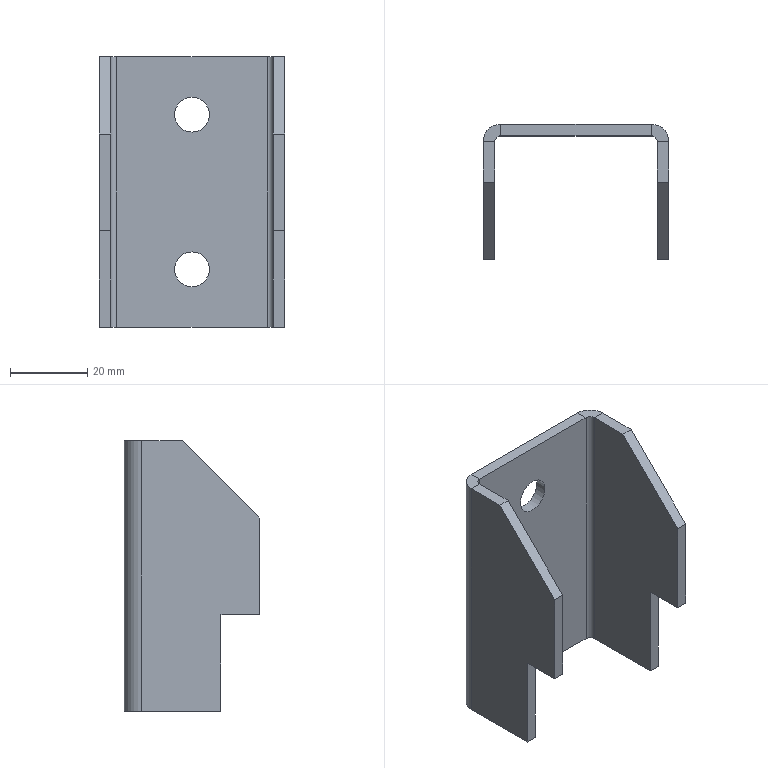Part | STEP file | 6150514 | 1 solid | 30 faces | box 48 x 35 x 70 mm | volume 19897 mm3 | plane 24 | cylinder 6 | commonest cylinder face diameters 9 x4 3 x2
STEP:
#1=CARTESIAN_POINT('',(-19.5,35.,35.));
#2=VERTEX_POINT('',#1);
#3=CARTESIAN_POINT('',(-19.5,32.,35.));
#4=VERTEX_POINT('',#3);
#5=CARTESIAN_POINT('',(-19.5,35.,35.));
#6=DIRECTION('',(0.,-1.,0.));
#7=VECTOR('',#6,1000.);
#8=LINE('',#5,#7);
#9=EDGE_CURVE('',#2,#4,#8,.T.);
#10=ORIENTED_EDGE('',*,*,#9,.F.);
#11=CARTESIAN_POINT('',(-24.,30.5,35.));
#12=VERTEX_POINT('',#11);
#13=CARTESIAN_POINT('',(-19.5,30.5,35.));
#14=DIRECTION('',(0.,0.,1.));
#15=DIRECTION('',(1.,0.,0.));
#16=AXIS2_PLACEMENT_3D('',#13,#14,#15);
#17=CIRCLE('',#16,4.5);
#18=EDGE_CURVE('',#2,#12,#17,.T.);
#19=ORIENTED_EDGE('',*,*,#18,.T.);
#20=CARTESIAN_POINT('',(-21.,30.5,35.));
#21=VERTEX_POINT('',#20);
#22=CARTESIAN_POINT('',(-21.,30.5,35.));
#23=DIRECTION('',(-1.,0.,0.));
#24=VECTOR('',#23,1000.);
#25=LINE('',#22,#24);
#26=EDGE_CURVE('',#21,#12,#25,.T.);
#27=ORIENTED_EDGE('',*,*,#26,.F.);
#28=CARTESIAN_POINT('',(-19.5,30.5,35.));
#29=DIRECTION('',(0.,0.,1.));
#30=DIRECTION('',(1.,0.,0.));
#31=AXIS2_PLACEMENT_3D('',#28,#29,#30);
#32=CIRCLE('',#31,1.5);
#33=EDGE_CURVE('',#4,#21,#32,.T.);
#34=ORIENTED_EDGE('',*,*,#33,.F.);
#35=EDGE_LOOP('',(#10,#19,#27,#34));
#36=FACE_OUTER_BOUND('',#35,.T.);
#37=CARTESIAN_POINT('',(-19.5,35.,35.));
#38=DIRECTION('',(0.,0.,1.));
#39=DIRECTION('',(1.,0.,0.));
#40=AXIS2_PLACEMENT_3D('',#37,#38,#39);
#41=PLANE('',#40);
#42=ADVANCED_FACE('',(#36),#41,.T.);
#43=CARTESIAN_POINT('',(19.5,35.,35.));
#44=VERTEX_POINT('',#43);
#45=CARTESIAN_POINT('',(-24.,35.,35.));
#46=DIRECTION('',(-1.,0.,0.));
#47=VECTOR('',#46,1000.);
#48=LINE('',#45,#47);
#49=EDGE_CURVE('',#44,#2,#48,.T.);
#50=ORIENTED_EDGE('',*,*,#49,.T.);
#51=ORIENTED_EDGE('',*,*,#9,.T.);
#52=CARTESIAN_POINT('',(19.5,32.,35.));
#53=VERTEX_POINT('',#52);
#54=CARTESIAN_POINT('',(-24.,32.,35.));
#55=DIRECTION('',(-1.,0.,0.));
#56=VECTOR('',#55,1000.);
#57=LINE('',#54,#56);
#58=EDGE_CURVE('',#53,#4,#57,.T.);
#59=ORIENTED_EDGE('',*,*,#58,.F.);
#60=CARTESIAN_POINT('',(19.5,32.,35.));
#61=DIRECTION('',(0.,1.,0.));
#62=VECTOR('',#61,1000.);
#63=LINE('',#60,#62);
#64=EDGE_CURVE('',#53,#44,#63,.T.);
#65=ORIENTED_EDGE('',*,*,#64,.T.);
#66=EDGE_LOOP('',(#50,#51,#59,#65));
#67=FACE_OUTER_BOUND('',#66,.T.);
#68=CARTESIAN_POINT('',(-21.,30.5,35.));
#69=DIRECTION('',(0.,0.,1.));
#70=DIRECTION('',(1.,0.,0.));
#71=AXIS2_PLACEMENT_3D('',#68,#69,#70);
#72=PLANE('',#71);
#73=ADVANCED_FACE('',(#67),#72,.T.);
#74=CARTESIAN_POINT('',(-24.,30.5,-35.));
#75=VERTEX_POINT('',#74);
#76=CARTESIAN_POINT('',(-21.,30.5,-35.));
#77=VERTEX_POINT('',#76);
#78=CARTESIAN_POINT('',(-24.,30.5,-35.));
#79=DIRECTION('',(1.,0.,0.));
#80=VECTOR('',#79,1000.);
#81=LINE('',#78,#80);
#82=EDGE_CURVE('',#75,#77,#81,.T.);
#83=ORIENTED_EDGE('',*,*,#82,.F.);
#84=CARTESIAN_POINT('',(-19.5,35.,-35.));
#85=VERTEX_POINT('',#84);
#86=CARTESIAN_POINT('',(-19.5,30.5,-35.));
#87=DIRECTION('',(0.,0.,1.));
#88=DIRECTION('',(1.,0.,0.));
#89=AXIS2_PLACEMENT_3D('',#86,#87,#88);
#90=CIRCLE('',#89,4.5);
#91=EDGE_CURVE('',#85,#75,#90,.T.);
#92=ORIENTED_EDGE('',*,*,#91,.F.);
#93=CARTESIAN_POINT('',(-19.5,32.,-35.));
#94=VERTEX_POINT('',#93);
#95=CARTESIAN_POINT('',(-19.5,32.,-35.));
#96=DIRECTION('',(0.,1.,0.));
#97=VECTOR('',#96,1000.);
#98=LINE('',#95,#97);
#99=EDGE_CURVE('',#94,#85,#98,.T.);
#100=ORIENTED_EDGE('',*,*,#99,.F.);
#101=CARTESIAN_POINT('',(-19.5,30.5,-35.));
#102=DIRECTION('',(0.,0.,1.));
#103=DIRECTION('',(1.,0.,0.));
#104=AXIS2_PLACEMENT_3D('',#101,#102,#103);
#105=CIRCLE('',#104,1.5);
#106=EDGE_CURVE('',#94,#77,#105,.T.);
#107=ORIENTED_EDGE('',*,*,#106,.T.);
#108=EDGE_LOOP('',(#83,#92,#100,#107));
#109=FACE_OUTER_BOUND('',#108,.T.);
#110=CARTESIAN_POINT('',(-24.,30.5,-35.));
#111=DIRECTION('',(0.,0.,-1.));
#112=DIRECTION('',(-1.,0.,0.));
#113=AXIS2_PLACEMENT_3D('',#110,#111,#112);
#114=PLANE('',#113);
#115=ADVANCED_FACE('',(#109),#114,.T.);
#116=CARTESIAN_POINT('',(-21.,10.,-35.));
#117=VERTEX_POINT('',#116);
#118=CARTESIAN_POINT('',(-24.,10.,-35.));
#119=VERTEX_POINT('',#118);
#120=CARTESIAN_POINT('',(24.,10.,-35.));
#121=DIRECTION('',(-1.,0.,0.));
#122=VECTOR('',#121,1000.);
#123=LINE('',#120,#122);
#124=EDGE_CURVE('',#117,#119,#123,.T.);
#125=ORIENTED_EDGE('',*,*,#124,.T.);
#126=CARTESIAN_POINT('',(-24.,0.,-35.));
#127=DIRECTION('',(0.,-1.,0.));
#128=VECTOR('',#127,1000.);
#129=LINE('',#126,#128);
#130=EDGE_CURVE('',#75,#119,#129,.T.);
#131=ORIENTED_EDGE('',*,*,#130,.F.);
#132=ORIENTED_EDGE('',*,*,#82,.T.);
#133=CARTESIAN_POINT('',(-21.,0.,-35.));
#134=DIRECTION('',(0.,-1.,0.));
#135=VECTOR('',#134,1000.);
#136=LINE('',#133,#135);
#137=EDGE_CURVE('',#77,#117,#136,.T.);
#138=ORIENTED_EDGE('',*,*,#137,.T.);
#139=EDGE_LOOP('',(#125,#131,#132,#138));
#140=FACE_OUTER_BOUND('',#139,.T.);
#141=CARTESIAN_POINT('',(-19.5,32.,-35.));
#142=DIRECTION('',(0.,0.,-1.));
#143=DIRECTION('',(-1.,0.,0.));
#144=AXIS2_PLACEMENT_3D('',#141,#142,#143);
#145=PLANE('',#144);
#146=ADVANCED_FACE('',(#140),#145,.T.);
#147=CARTESIAN_POINT('',(24.,30.5,35.));
#148=VERTEX_POINT('',#147);
#149=CARTESIAN_POINT('',(21.,30.5,35.));
#150=VERTEX_POINT('',#149);
#151=CARTESIAN_POINT('',(24.,30.5,35.));
#152=DIRECTION('',(-1.,0.,0.));
#153=VECTOR('',#152,1000.);
#154=LINE('',#151,#153);
#155=EDGE_CURVE('',#148,#150,#154,.T.);
#156=ORIENTED_EDGE('',*,*,#155,.F.);
#157=CARTESIAN_POINT('',(19.5,30.5,35.));
#158=DIRECTION('',(0.,0.,1.));
#159=DIRECTION('',(1.,0.,0.));
#160=AXIS2_PLACEMENT_3D('',#157,#158,#159);
#161=CIRCLE('',#160,4.5);
#162=EDGE_CURVE('',#148,#44,#161,.T.);
#163=ORIENTED_EDGE('',*,*,#162,.T.);
#164=ORIENTED_EDGE('',*,*,#64,.F.);
#165=CARTESIAN_POINT('',(19.5,30.5,35.));
#166=DIRECTION('',(0.,0.,1.));
#167=DIRECTION('',(1.,0.,0.));
#168=AXIS2_PLACEMENT_3D('',#165,#166,#167);
#169=CIRCLE('',#168,1.5);
#170=EDGE_CURVE('',#150,#53,#169,.T.);
#171=ORIENTED_EDGE('',*,*,#170,.F.);
#172=EDGE_LOOP('',(#156,#163,#164,#171));
#173=FACE_OUTER_BOUND('',#172,.T.);
#174=CARTESIAN_POINT('',(24.,30.5,35.));
#175=DIRECTION('',(0.,0.,1.));
#176=DIRECTION('',(1.,0.,0.));
#177=AXIS2_PLACEMENT_3D('',#174,#175,#176);
#178=PLANE('',#177);
#179=ADVANCED_FACE('',(#173),#178,.T.);
#180=CARTESIAN_POINT('',(21.,20.,35.));
#181=VERTEX_POINT('',#180);
#182=CARTESIAN_POINT('',(24.,20.,35.));
#183=VERTEX_POINT('',#182);
#184=CARTESIAN_POINT('',(-144.387,20.,35.));
#185=DIRECTION('',(1.,0.,0.));
#186=VECTOR('',#185,1000.);
#187=LINE('',#184,#186);
#188=EDGE_CURVE('',#181,#183,#187,.T.);
#189=ORIENTED_EDGE('',*,*,#188,.T.);
#190=CARTESIAN_POINT('',(24.,0.,35.));
#191=DIRECTION('',(0.,1.,0.));
#192=VECTOR('',#191,1000.);
#193=LINE('',#190,#192);
#194=EDGE_CURVE('',#183,#148,#193,.T.);
#195=ORIENTED_EDGE('',*,*,#194,.T.);
#196=ORIENTED_EDGE('',*,*,#155,.T.);
#197=CARTESIAN_POINT('',(21.,0.,35.));
#198=DIRECTION('',(0.,1.,0.));
#199=VECTOR('',#198,1000.);
#200=LINE('',#197,#199);
#201=EDGE_CURVE('',#181,#150,#200,.T.);
#202=ORIENTED_EDGE('',*,*,#201,.F.);
#203=EDGE_LOOP('',(#189,#195,#196,#202));
#204=FACE_OUTER_BOUND('',#203,.T.);
#205=CARTESIAN_POINT('',(19.5,32.,35.));
#206=DIRECTION('',(0.,0.,1.));
#207=DIRECTION('',(1.,0.,0.));
#208=AXIS2_PLACEMENT_3D('',#205,#206,#207);
#209=PLANE('',#208);
#210=ADVANCED_FACE('',(#204),#209,.T.);
#211=CARTESIAN_POINT('',(19.5,35.,-35.));
#212=VERTEX_POINT('',#211);
#213=CARTESIAN_POINT('',(19.5,32.,-35.));
#214=VERTEX_POINT('',#213);
#215=CARTESIAN_POINT('',(19.5,35.,-35.));
#216=DIRECTION('',(0.,-1.,0.));
#217=VECTOR('',#216,1000.);
#218=LINE('',#215,#217);
#219=EDGE_CURVE('',#212,#214,#218,.T.);
#220=ORIENTED_EDGE('',*,*,#219,.F.);
#221=CARTESIAN_POINT('',(24.,30.5,-35.));
#222=VERTEX_POINT('',#221);
#223=CARTESIAN_POINT('',(19.5,30.5,-35.));
#224=DIRECTION('',(0.,0.,1.));
#225=DIRECTION('',(1.,0.,0.));
#226=AXIS2_PLACEMENT_3D('',#223,#224,#225);
#227=CIRCLE('',#226,4.5);
#228=EDGE_CURVE('',#222,#212,#227,.T.);
#229=ORIENTED_EDGE('',*,*,#228,.F.);
#230=CARTESIAN_POINT('',(21.,30.5,-35.));
#231=VERTEX_POINT('',#230);
#232=CARTESIAN_POINT('',(21.,30.5,-35.));
#233=DIRECTION('',(1.,0.,0.));
#234=VECTOR('',#233,1000.);
#235=LINE('',#232,#234);
#236=EDGE_CURVE('',#231,#222,#235,.T.);
#237=ORIENTED_EDGE('',*,*,#236,.F.);
#238=CARTESIAN_POINT('',(19.5,30.5,-35.));
#239=DIRECTION('',(0.,0.,1.));
#240=DIRECTION('',(1.,0.,0.));
#241=AXIS2_PLACEMENT_3D('',#238,#239,#240);
#242=CIRCLE('',#241,1.5);
#243=EDGE_CURVE('',#231,#214,#242,.T.);
#244=ORIENTED_EDGE('',*,*,#243,.T.);
#245=EDGE_LOOP('',(#220,#229,#237,#244));
#246=FACE_OUTER_BOUND('',#245,.T.);
#247=CARTESIAN_POINT('',(19.5,35.,-35.));
#248=DIRECTION('',(0.,0.,-1.));
#249=DIRECTION('',(-1.,0.,0.));
#250=AXIS2_PLACEMENT_3D('',#247,#248,#249);
#251=PLANE('',#250);
#252=ADVANCED_FACE('',(#246),#251,.T.);
#253=CARTESIAN_POINT('',(-24.,35.,-35.));
#254=DIRECTION('',(-1.,0.,0.));
#255=VECTOR('',#254,1000.);
#256=LINE('',#253,#255);
#257=EDGE_CURVE('',#212,#85,#256,.T.);
#258=ORIENTED_EDGE('',*,*,#257,.F.);
#259=ORIENTED_EDGE('',*,*,#219,.T.);
#260=CARTESIAN_POINT('',(-24.,32.,-35.));
#261=DIRECTION('',(-1.,0.,0.));
#262=VECTOR('',#261,1000.);
#263=LINE('',#260,#262);
#264=EDGE_CURVE('',#214,#94,#263,.T.);
#265=ORIENTED_EDGE('',*,*,#264,.T.);
#266=ORIENTED_EDGE('',*,*,#99,.T.);
#267=EDGE_LOOP('',(#258,#259,#265,#266));
#268=FACE_OUTER_BOUND('',#267,.T.);
#269=CARTESIAN_POINT('',(21.,30.5,-35.));
#270=DIRECTION('',(0.,0.,-1.));
#271=DIRECTION('',(-1.,0.,0.));
#272=AXIS2_PLACEMENT_3D('',#269,#270,#271);
#273=PLANE('',#272);
#274=ADVANCED_FACE('',(#268),#273,.T.);
#275=ORIENTED_EDGE('',*,*,#130,.T.);
#276=CARTESIAN_POINT('',(-24.,10.,-10.));
#277=VERTEX_POINT('',#276);
#278=CARTESIAN_POINT('',(-24.,10.,-35.));
#279=DIRECTION('',(0.,0.,-1.));
#280=VECTOR('',#279,1000.);
#281=LINE('',#278,#280);
#282=EDGE_CURVE('',#277,#119,#281,.T.);
#283=ORIENTED_EDGE('',*,*,#282,.F.);
#284=CARTESIAN_POINT('',(-24.,0.,-10.));
#285=VERTEX_POINT('',#284);
#286=CARTESIAN_POINT('',(-24.,10.,-10.));
#287=DIRECTION('',(0.,1.,0.));
#288=VECTOR('',#287,1000.);
#289=LINE('',#286,#288);
#290=EDGE_CURVE('',#285,#277,#289,.T.);
#291=ORIENTED_EDGE('',*,*,#290,.F.);
#292=CARTESIAN_POINT('',(-24.,0.,15.));
#293=VERTEX_POINT('',#292);
#294=CARTESIAN_POINT('',(-24.,0.,35.));
#295=DIRECTION('',(0.,0.,-1.));
#296=VECTOR('',#295,1000.);
#297=LINE('',#294,#296);
#298=EDGE_CURVE('',#293,#285,#297,.T.);
#299=ORIENTED_EDGE('',*,*,#298,.F.);
#300=CARTESIAN_POINT('',(-24.,20.,35.));
#301=VERTEX_POINT('',#300);
#302=CARTESIAN_POINT('',(-24.,10.,25.));
#303=DIRECTION('',(0.,0.7071,0.7071));
#304=VECTOR('',#303,1000.);
#305=LINE('',#302,#304);
#306=EDGE_CURVE('',#293,#301,#305,.T.);
#307=ORIENTED_EDGE('',*,*,#306,.T.);
#308=CARTESIAN_POINT('',(-24.,0.,35.));
#309=DIRECTION('',(0.,-1.,0.));
#310=VECTOR('',#309,1000.);
#311=LINE('',#308,#310);
#312=EDGE_CURVE('',#12,#301,#311,.T.);
#313=ORIENTED_EDGE('',*,*,#312,.F.);
#314=CARTESIAN_POINT('',(-24.,30.5,35.));
#315=DIRECTION('',(0.,0.,-1.));
#316=VECTOR('',#315,1000.);
#317=LINE('',#314,#316);
#318=EDGE_CURVE('',#12,#75,#317,.T.);
#319=ORIENTED_EDGE('',*,*,#318,.T.);
#320=EDGE_LOOP('',(#275,#283,#291,#299,#307,#313,#319));
#321=FACE_OUTER_BOUND('',#320,.T.);
#322=CARTESIAN_POINT('',(-24.,0.,35.));
#323=DIRECTION('',(1.,0.,0.));
#324=DIRECTION('',(0.,0.,-1.));
#325=AXIS2_PLACEMENT_3D('',#322,#323,#324);
#326=PLANE('',#325);
#327=ADVANCED_FACE('',(#321),#326,.F.);
#328=CARTESIAN_POINT('',(-21.,0.,-10.));
#329=VERTEX_POINT('',#328);
#330=CARTESIAN_POINT('',(24.,0.,-10.));
#331=DIRECTION('',(-1.,0.,0.));
#332=VECTOR('',#331,1000.);
#333=LINE('',#330,#332);
#334=EDGE_CURVE('',#329,#285,#333,.T.);
#335=ORIENTED_EDGE('',*,*,#334,.F.);
#336=CARTESIAN_POINT('',(-21.,0.,15.));
#337=VERTEX_POINT('',#336);
#338=CARTESIAN_POINT('',(-21.,0.,35.));
#339=DIRECTION('',(0.,0.,-1.));
#340=VECTOR('',#339,1000.);
#341=LINE('',#338,#340);
#342=EDGE_CURVE('',#337,#329,#341,.T.);
#343=ORIENTED_EDGE('',*,*,#342,.F.);
#344=CARTESIAN_POINT('',(-144.387,0.,15.));
#345=DIRECTION('',(1.,0.,0.));
#346=VECTOR('',#345,1000.);
#347=LINE('',#344,#346);
#348=EDGE_CURVE('',#293,#337,#347,.T.);
#349=ORIENTED_EDGE('',*,*,#348,.F.);
#350=ORIENTED_EDGE('',*,*,#298,.T.);
#351=EDGE_LOOP('',(#335,#343,#349,#350));
#352=FACE_OUTER_BOUND('',#351,.T.);
#353=CARTESIAN_POINT('',(-21.,0.,35.));
#354=DIRECTION('',(0.,-1.,0.));
#355=DIRECTION('',(0.,0.,-1.));
#356=AXIS2_PLACEMENT_3D('',#353,#354,#355);
#357=PLANE('',#356);
#358=ADVANCED_FACE('',(#352),#357,.T.);
#359=CARTESIAN_POINT('',(-21.,10.,-10.));
#360=VERTEX_POINT('',#359);
#361=CARTESIAN_POINT('',(-21.,10.,35.));
#362=DIRECTION('',(0.,0.,1.));
#363=VECTOR('',#362,1000.);
#364=LINE('',#361,#363);
#365=EDGE_CURVE('',#117,#360,#364,.T.);
#366=ORIENTED_EDGE('',*,*,#365,.F.);
#367=ORIENTED_EDGE('',*,*,#137,.F.);
#368=CARTESIAN_POINT('',(-21.,30.5,35.));
#369=DIRECTION('',(0.,0.,-1.));
#370=VECTOR('',#369,1000.);
#371=LINE('',#368,#370);
#372=EDGE_CURVE('',#21,#77,#371,.T.);
#373=ORIENTED_EDGE('',*,*,#372,.F.);
#374=CARTESIAN_POINT('',(-21.,20.,35.));
#375=VERTEX_POINT('',#374);
#376=CARTESIAN_POINT('',(-21.,0.,35.));
#377=DIRECTION('',(0.,-1.,0.));
#378=VECTOR('',#377,1000.);
#379=LINE('',#376,#378);
#380=EDGE_CURVE('',#21,#375,#379,.T.);
#381=ORIENTED_EDGE('',*,*,#380,.T.);
#382=CARTESIAN_POINT('',(-21.,10.,25.));
#383=DIRECTION('',(0.,0.7071,0.7071));
#384=VECTOR('',#383,1000.);
#385=LINE('',#382,#384);
#386=EDGE_CURVE('',#337,#375,#385,.T.);
#387=ORIENTED_EDGE('',*,*,#386,.F.);
#388=ORIENTED_EDGE('',*,*,#342,.T.);
#389=CARTESIAN_POINT('',(-21.,0.,-10.));
#390=DIRECTION('',(0.,-1.,0.));
#391=VECTOR('',#390,1000.);
#392=LINE('',#389,#391);
#393=EDGE_CURVE('',#360,#329,#392,.T.);
#394=ORIENTED_EDGE('',*,*,#393,.F.);
#395=EDGE_LOOP('',(#366,#367,#373,#381,#387,#388,#394));
#396=FACE_OUTER_BOUND('',#395,.T.);
#397=CARTESIAN_POINT('',(-21.,0.,35.));
#398=DIRECTION('',(1.,0.,0.));
#399=DIRECTION('',(0.,0.,-1.));
#400=AXIS2_PLACEMENT_3D('',#397,#398,#399);
#401=PLANE('',#400);
#402=ADVANCED_FACE('',(#396),#401,.T.);
#403=ORIENTED_EDGE('',*,*,#106,.F.);
#404=CARTESIAN_POINT('',(-19.5,32.,35.));
#405=DIRECTION('',(0.,0.,-1.));
#406=VECTOR('',#405,1000.);
#407=LINE('',#404,#406);
#408=EDGE_CURVE('',#4,#94,#407,.T.);
#409=ORIENTED_EDGE('',*,*,#408,.F.);
#410=ORIENTED_EDGE('',*,*,#33,.T.);
#411=ORIENTED_EDGE('',*,*,#372,.T.);
#412=EDGE_LOOP('',(#403,#409,#410,#411));
#413=FACE_OUTER_BOUND('',#412,.T.);
#414=CARTESIAN_POINT('',(-19.5,30.5,35.));
#415=DIRECTION('',(0.,0.,-1.));
#416=DIRECTION('',(-1.,0.,0.));
#417=AXIS2_PLACEMENT_3D('',#414,#415,#416);
#418=CYLINDRICAL_SURFACE('',#417,1.5);
#419=ADVANCED_FACE('',(#413),#418,.F.);
#420=CARTESIAN_POINT('',(0.,32.,15.5));
#421=VERTEX_POINT('',#420);
#422=CARTESIAN_POINT('',(0.,32.,20.));
#423=DIRECTION('',(0.,-1.,0.));
#424=DIRECTION('',(0.,0.,-1.));
#425=AXIS2_PLACEMENT_3D('',#422,#423,#424);
#426=CIRCLE('',#425,4.5);
#427=EDGE_CURVE('',#421,#421,#426,.T.);
#428=ORIENTED_EDGE('',*,*,#427,.F.);
#429=EDGE_LOOP('',(#428));
#430=FACE_BOUND('',#429,.T.);
#431=CARTESIAN_POINT('',(0.,32.,-24.5));
#432=VERTEX_POINT('',#431);
#433=CARTESIAN_POINT('',(0.,32.,-20.));
#434=DIRECTION('',(0.,-1.,0.));
#435=DIRECTION('',(0.,0.,-1.));
#436=AXIS2_PLACEMENT_3D('',#433,#434,#435);
#437=CIRCLE('',#436,4.5);
#438=EDGE_CURVE('',#432,#432,#437,.T.);
#439=ORIENTED_EDGE('',*,*,#438,.F.);
#440=EDGE_LOOP('',(#439));
#441=FACE_BOUND('',#440,.T.);
#442=ORIENTED_EDGE('',*,*,#264,.F.);
#443=CARTESIAN_POINT('',(19.5,32.,35.));
#444=DIRECTION('',(0.,0.,-1.));
#445=VECTOR('',#444,1000.);
#446=LINE('',#443,#445);
#447=EDGE_CURVE('',#53,#214,#446,.T.);
#448=ORIENTED_EDGE('',*,*,#447,.F.);
#449=ORIENTED_EDGE('',*,*,#58,.T.);
#450=ORIENTED_EDGE('',*,*,#408,.T.);
#451=EDGE_LOOP('',(#442,#448,#449,#450));
#452=FACE_OUTER_BOUND('',#451,.T.);
#453=CARTESIAN_POINT('',(-24.,32.,35.));
#454=DIRECTION('',(0.,-1.,0.));
#455=DIRECTION('',(0.,0.,-1.));
#456=AXIS2_PLACEMENT_3D('',#453,#454,#455);
#457=PLANE('',#456);
#458=ADVANCED_FACE('',(#430,#441,#452),#457,.T.);
#459=ORIENTED_EDGE('',*,*,#243,.F.);
#460=CARTESIAN_POINT('',(21.,30.5,35.));
#461=DIRECTION('',(0.,0.,-1.));
#462=VECTOR('',#461,1000.);
#463=LINE('',#460,#462);
#464=EDGE_CURVE('',#150,#231,#463,.T.);
#465=ORIENTED_EDGE('',*,*,#464,.F.);
#466=ORIENTED_EDGE('',*,*,#170,.T.);
#467=ORIENTED_EDGE('',*,*,#447,.T.);
#468=EDGE_LOOP('',(#459,#465,#466,#467));
#469=FACE_OUTER_BOUND('',#468,.T.);
#470=CARTESIAN_POINT('',(19.5,30.5,35.));
#471=DIRECTION('',(0.,0.,-1.));
#472=DIRECTION('',(-1.,0.,0.));
#473=AXIS2_PLACEMENT_3D('',#470,#471,#472);
#474=CYLINDRICAL_SURFACE('',#473,1.5);
#475=ADVANCED_FACE('',(#469),#474,.F.);
#476=CARTESIAN_POINT('',(21.,10.,-10.));
#477=VERTEX_POINT('',#476);
#478=CARTESIAN_POINT('',(21.,10.,-35.));
#479=VERTEX_POINT('',#478);
#480=CARTESIAN_POINT('',(21.,10.,35.));
#481=DIRECTION('',(0.,0.,-1.));
#482=VECTOR('',#481,1000.);
#483=LINE('',#480,#482);
#484=EDGE_CURVE('',#477,#479,#483,.T.);
#485=ORIENTED_EDGE('',*,*,#484,.F.);
#486=CARTESIAN_POINT('',(21.,0.,-10.));
#487=VERTEX_POINT('',#486);
#488=CARTESIAN_POINT('',(21.,0.,-10.));
#489=DIRECTION('',(0.,1.,0.));
#490=VECTOR('',#489,1000.);
#491=LINE('',#488,#490);
#492=EDGE_CURVE('',#487,#477,#491,.T.);
#493=ORIENTED_EDGE('',*,*,#492,.F.);
#494=CARTESIAN_POINT('',(21.,0.,15.));
#495=VERTEX_POINT('',#494);
#496=CARTESIAN_POINT('',(21.,0.,35.));
#497=DIRECTION('',(0.,0.,-1.));
#498=VECTOR('',#497,1000.);
#499=LINE('',#496,#498);
#500=EDGE_CURVE('',#495,#487,#499,.T.);
#501=ORIENTED_EDGE('',*,*,#500,.F.);
#502=CARTESIAN_POINT('',(21.,10.,25.));
#503=DIRECTION('',(0.,-0.7071,-0.7071));
#504=VECTOR('',#503,1000.);
#505=LINE('',#502,#504);
#506=EDGE_CURVE('',#181,#495,#505,.T.);
#507=ORIENTED_EDGE('',*,*,#506,.F.);
#508=ORIENTED_EDGE('',*,*,#201,.T.);
#509=ORIENTED_EDGE('',*,*,#464,.T.);
#510=CARTESIAN_POINT('',(21.,0.,-35.));
#511=DIRECTION('',(0.,1.,0.));
#512=VECTOR('',#511,1000.);
#513=LINE('',#510,#512);
#514=EDGE_CURVE('',#479,#231,#513,.T.);
#515=ORIENTED_EDGE('',*,*,#514,.F.);
#516=EDGE_LOOP('',(#485,#493,#501,#507,#508,#509,#515));
#517=FACE_OUTER_BOUND('',#516,.T.);
#518=CARTESIAN_POINT('',(21.,0.,35.));
#519=DIRECTION('',(-1.,0.,0.));
#520=DIRECTION('',(0.,0.,1.));
#521=AXIS2_PLACEMENT_3D('',#518,#519,#520);
#522=PLANE('',#521);
#523=ADVANCED_FACE('',(#517),#522,.T.);
#524=CARTESIAN_POINT('',(24.,0.,-10.));
#525=VERTEX_POINT('',#524);
#526=CARTESIAN_POINT('',(24.,0.,-10.));
#527=DIRECTION('',(-1.,0.,0.));
#528=VECTOR('',#527,1000.);
#529=LINE('',#526,#528);
#530=EDGE_CURVE('',#525,#487,#529,.T.);
#531=ORIENTED_EDGE('',*,*,#530,.F.);
#532=CARTESIAN_POINT('',(24.,0.,15.));
#533=VERTEX_POINT('',#532);
#534=CARTESIAN_POINT('',(24.,0.,35.));
#535=DIRECTION('',(0.,0.,-1.));
#536=VECTOR('',#535,1000.);
#537=LINE('',#534,#536);
#538=EDGE_CURVE('',#533,#525,#537,.T.);
#539=ORIENTED_EDGE('',*,*,#538,.F.);
#540=CARTESIAN_POINT('',(-144.387,0.,15.));
#541=DIRECTION('',(1.,0.,0.));
#542=VECTOR('',#541,1000.);
#543=LINE('',#540,#542);
#544=EDGE_CURVE('',#495,#533,#543,.T.);
#545=ORIENTED_EDGE('',*,*,#544,.F.);
#546=ORIENTED_EDGE('',*,*,#500,.T.);
#547=EDGE_LOOP('',(#531,#539,#545,#546));
#548=FACE_OUTER_BOUND('',#547,.T.);
#549=CARTESIAN_POINT('',(24.,0.,35.));
#550=DIRECTION('',(0.,-1.,0.));
#551=DIRECTION('',(0.,0.,-1.));
#552=AXIS2_PLACEMENT_3D('',#549,#550,#551);
#553=PLANE('',#552);
#554=ADVANCED_FACE('',(#548),#553,.T.);
#555=CARTESIAN_POINT('',(24.,10.,-10.));
#556=VERTEX_POINT('',#555);
#557=CARTESIAN_POINT('',(24.,10.,-10.));
#558=DIRECTION('',(0.,1.,0.));
#559=VECTOR('',#558,1000.);
#560=LINE('',#557,#559);
#561=EDGE_CURVE('',#525,#556,#560,.T.);
#562=ORIENTED_EDGE('',*,*,#561,.T.);
#563=CARTESIAN_POINT('',(24.,10.,-35.));
#564=VERTEX_POINT('',#563);
#565=CARTESIAN_POINT('',(24.,10.,-35.));
#566=DIRECTION('',(0.,0.,-1.));
#567=VECTOR('',#566,1000.);
#568=LINE('',#565,#567);
#569=EDGE_CURVE('',#556,#564,#568,.T.);
#570=ORIENTED_EDGE('',*,*,#569,.T.);
#571=CARTESIAN_POINT('',(24.,0.,-35.));
#572=DIRECTION('',(0.,1.,0.));
#573=VECTOR('',#572,1000.);
#574=LINE('',#571,#573);
#575=EDGE_CURVE('',#564,#222,#574,.T.);
#576=ORIENTED_EDGE('',*,*,#575,.T.);
#577=CARTESIAN_POINT('',(24.,30.5,35.));
#578=DIRECTION('',(0.,0.,-1.));
#579=VECTOR('',#578,1000.);
#580=LINE('',#577,#579);
#581=EDGE_CURVE('',#148,#222,#580,.T.);
#582=ORIENTED_EDGE('',*,*,#581,.F.);
#583=ORIENTED_EDGE('',*,*,#194,.F.);
#584=CARTESIAN_POINT('',(24.,10.,25.));
#585=DIRECTION('',(0.,-0.7071,-0.7071));
#586=VECTOR('',#585,1000.);
#587=LINE('',#584,#586);
#588=EDGE_CURVE('',#183,#533,#587,.T.);
#589=ORIENTED_EDGE('',*,*,#588,.T.);
#590=ORIENTED_EDGE('',*,*,#538,.T.);
#591=EDGE_LOOP('',(#562,#570,#576,#582,#583,#589,#590));
#592=FACE_OUTER_BOUND('',#591,.T.);
#593=CARTESIAN_POINT('',(24.,0.,35.));
#594=DIRECTION('',(-1.,0.,0.));
#595=DIRECTION('',(0.,0.,1.));
#596=AXIS2_PLACEMENT_3D('',#593,#594,#595);
#597=PLANE('',#596);
#598=ADVANCED_FACE('',(#592),#597,.F.);
#599=ORIENTED_EDGE('',*,*,#228,.T.);
#600=CARTESIAN_POINT('',(19.5,35.,35.));
#601=DIRECTION('',(0.,0.,-1.));
#602=VECTOR('',#601,1000.);
#603=LINE('',#600,#602);
#604=EDGE_CURVE('',#44,#212,#603,.T.);
#605=ORIENTED_EDGE('',*,*,#604,.F.);
#606=ORIENTED_EDGE('',*,*,#162,.F.);
#607=ORIENTED_EDGE('',*,*,#581,.T.);
#608=EDGE_LOOP('',(#599,#605,#606,#607));
#609=FACE_OUTER_BOUND('',#608,.T.);
#610=CARTESIAN_POINT('',(19.5,30.5,35.));
#611=DIRECTION('',(0.,0.,-1.));
#612=DIRECTION('',(-1.,0.,0.));
#613=AXIS2_PLACEMENT_3D('',#610,#611,#612);
#614=CYLINDRICAL_SURFACE('',#613,4.5);
#615=ADVANCED_FACE('',(#609),#614,.T.);
#616=CARTESIAN_POINT('',(0.,35.,24.5));
#617=VERTEX_POINT('',#616);
#618=CARTESIAN_POINT('',(0.,35.,20.));
#619=DIRECTION('',(0.,1.,0.));
#620=DIRECTION('',(0.,0.,1.));
#621=AXIS2_PLACEMENT_3D('',#618,#619,#620);
#622=CIRCLE('',#621,4.5);
#623=EDGE_CURVE('',#617,#617,#622,.T.);
#624=ORIENTED_EDGE('',*,*,#623,.F.);
#625=EDGE_LOOP('',(#624));
#626=FACE_BOUND('',#625,.T.);
#627=CARTESIAN_POINT('',(0.,35.,-15.5));
#628=VERTEX_POINT('',#627);
#629=CARTESIAN_POINT('',(0.,35.,-20.));
#630=DIRECTION('',(0.,1.,0.));
#631=DIRECTION('',(0.,0.,1.));
#632=AXIS2_PLACEMENT_3D('',#629,#630,#631);
#633=CIRCLE('',#632,4.5);
#634=EDGE_CURVE('',#628,#628,#633,.T.);
#635=ORIENTED_EDGE('',*,*,#634,.F.);
#636=EDGE_LOOP('',(#635));
#637=FACE_BOUND('',#636,.T.);
#638=ORIENTED_EDGE('',*,*,#257,.T.);
#639=CARTESIAN_POINT('',(-19.5,35.,35.));
#640=DIRECTION('',(0.,0.,-1.));
#641=VECTOR('',#640,1000.);
#642=LINE('',#639,#641);
#643=EDGE_CURVE('',#2,#85,#642,.T.);
#644=ORIENTED_EDGE('',*,*,#643,.F.);
#645=ORIENTED_EDGE('',*,*,#49,.F.);
#646=ORIENTED_EDGE('',*,*,#604,.T.);
#647=EDGE_LOOP('',(#638,#644,#645,#646));
#648=FACE_OUTER_BOUND('',#647,.T.);
#649=CARTESIAN_POINT('',(-24.,35.,35.));
#650=DIRECTION('',(0.,-1.,0.));
#651=DIRECTION('',(0.,0.,-1.));
#652=AXIS2_PLACEMENT_3D('',#649,#650,#651);
#653=PLANE('',#652);
#654=ADVANCED_FACE('',(#626,#637,#648),#653,.F.);
#655=ORIENTED_EDGE('',*,*,#91,.T.);
#656=ORIENTED_EDGE('',*,*,#318,.F.);
#657=ORIENTED_EDGE('',*,*,#18,.F.);
#658=ORIENTED_EDGE('',*,*,#643,.T.);
#659=EDGE_LOOP('',(#655,#656,#657,#658));
#660=FACE_OUTER_BOUND('',#659,.T.);
#661=CARTESIAN_POINT('',(-19.5,30.5,35.));
#662=DIRECTION('',(0.,0.,-1.));
#663=DIRECTION('',(-1.,0.,0.));
#664=AXIS2_PLACEMENT_3D('',#661,#662,#663);
#665=CYLINDRICAL_SURFACE('',#664,4.5);
#666=ADVANCED_FACE('',(#660),#665,.T.);
#667=CARTESIAN_POINT('',(-19.5,20.,35.));
#668=DIRECTION('',(-1.,0.,0.));
#669=VECTOR('',#668,1000.);
#670=LINE('',#667,#669);
#671=EDGE_CURVE('',#375,#301,#670,.T.);
#672=ORIENTED_EDGE('',*,*,#671,.F.);
#673=ORIENTED_EDGE('',*,*,#380,.F.);
#674=ORIENTED_EDGE('',*,*,#26,.T.);
#675=ORIENTED_EDGE('',*,*,#312,.T.);
#676=EDGE_LOOP('',(#672,#673,#674,#675));
#677=FACE_OUTER_BOUND('',#676,.T.);
#678=CARTESIAN_POINT('',(-19.5,30.5,35.));
#679=DIRECTION('',(0.,0.,1.));
#680=DIRECTION('',(1.,0.,0.));
#681=AXIS2_PLACEMENT_3D('',#678,#679,#680);
#682=PLANE('',#681);
#683=ADVANCED_FACE('',(#677),#682,.T.);
#684=ORIENTED_EDGE('',*,*,#575,.F.);
#685=CARTESIAN_POINT('',(24.,10.,-35.));
#686=DIRECTION('',(-1.,0.,0.));
#687=VECTOR('',#686,1000.);
#688=LINE('',#685,#687);
#689=EDGE_CURVE('',#564,#479,#688,.T.);
#690=ORIENTED_EDGE('',*,*,#689,.T.);
#691=ORIENTED_EDGE('',*,*,#514,.T.);
#692=ORIENTED_EDGE('',*,*,#236,.T.);
#693=EDGE_LOOP('',(#684,#690,#691,#692));
#694=FACE_OUTER_BOUND('',#693,.T.);
#695=CARTESIAN_POINT('',(-19.5,30.5,-35.));
#696=DIRECTION('',(0.,0.,1.));
#697=DIRECTION('',(1.,0.,0.));
#698=AXIS2_PLACEMENT_3D('',#695,#696,#697);
#699=PLANE('',#698);
#700=ADVANCED_FACE('',(#694),#699,.F.);
#701=ORIENTED_EDGE('',*,*,#306,.F.);
#702=ORIENTED_EDGE('',*,*,#348,.T.);
#703=ORIENTED_EDGE('',*,*,#386,.T.);
#704=ORIENTED_EDGE('',*,*,#671,.T.);
#705=EDGE_LOOP('',(#701,#702,#703,#704));
#706=FACE_OUTER_BOUND('',#705,.T.);
#707=CARTESIAN_POINT('',(-144.387,0.,15.));
#708=DIRECTION('',(0.,0.7071,-0.7071));
#709=DIRECTION('',(0.,0.7071,0.7071));
#710=AXIS2_PLACEMENT_3D('',#707,#708,#709);
#711=PLANE('',#710);
#712=ADVANCED_FACE('',(#706),#711,.F.);
#713=ORIENTED_EDGE('',*,*,#188,.F.);
#714=ORIENTED_EDGE('',*,*,#506,.T.);
#715=ORIENTED_EDGE('',*,*,#544,.T.);
#716=ORIENTED_EDGE('',*,*,#588,.F.);
#717=EDGE_LOOP('',(#713,#714,#715,#716));
#718=FACE_OUTER_BOUND('',#717,.T.);
#719=CARTESIAN_POINT('',(-144.387,0.,15.));
#720=DIRECTION('',(0.,0.7071,-0.7071));
#721=DIRECTION('',(0.,0.7071,0.7071));
#722=AXIS2_PLACEMENT_3D('',#719,#720,#721);
#723=PLANE('',#722);
#724=ADVANCED_FACE('',(#718),#723,.F.);
#725=ORIENTED_EDGE('',*,*,#484,.T.);
#726=ORIENTED_EDGE('',*,*,#689,.F.);
#727=ORIENTED_EDGE('',*,*,#569,.F.);
#728=CARTESIAN_POINT('',(24.,10.,-10.));
#729=DIRECTION('',(-1.,0.,0.));
#730=VECTOR('',#729,1000.);
#731=LINE('',#728,#730);
#732=EDGE_CURVE('',#556,#477,#731,.T.);
#733=ORIENTED_EDGE('',*,*,#732,.T.);
#734=EDGE_LOOP('',(#725,#726,#727,#733));
#735=FACE_OUTER_BOUND('',#734,.T.);
#736=CARTESIAN_POINT('',(24.,10.,-35.));
#737=DIRECTION('',(0.,1.,0.));
#738=DIRECTION('',(0.,0.,1.));
#739=AXIS2_PLACEMENT_3D('',#736,#737,#738);
#740=PLANE('',#739);
#741=ADVANCED_FACE('',(#735),#740,.F.);
#742=ORIENTED_EDGE('',*,*,#492,.T.);
#743=ORIENTED_EDGE('',*,*,#732,.F.);
#744=ORIENTED_EDGE('',*,*,#561,.F.);
#745=ORIENTED_EDGE('',*,*,#530,.T.);
#746=EDGE_LOOP('',(#742,#743,#744,#745));
#747=FACE_OUTER_BOUND('',#746,.T.);
#748=CARTESIAN_POINT('',(24.,10.,-10.));
#749=DIRECTION('',(0.,0.,1.));
#750=DIRECTION('',(0.,-1.,0.));
#751=AXIS2_PLACEMENT_3D('',#748,#749,#750);
#752=PLANE('',#751);
#753=ADVANCED_FACE('',(#747),#752,.F.);
#754=ORIENTED_EDGE('',*,*,#393,.T.);
#755=ORIENTED_EDGE('',*,*,#334,.T.);
#756=ORIENTED_EDGE('',*,*,#290,.T.);
#757=CARTESIAN_POINT('',(24.,10.,-10.));
#758=DIRECTION('',(-1.,0.,0.));
#759=VECTOR('',#758,1000.);
#760=LINE('',#757,#759);
#761=EDGE_CURVE('',#360,#277,#760,.T.);
#762=ORIENTED_EDGE('',*,*,#761,.F.);
#763=EDGE_LOOP('',(#754,#755,#756,#762));
#764=FACE_OUTER_BOUND('',#763,.T.);
#765=CARTESIAN_POINT('',(24.,10.,-10.));
#766=DIRECTION('',(0.,0.,1.));
#767=DIRECTION('',(0.,-1.,0.));
#768=AXIS2_PLACEMENT_3D('',#765,#766,#767);
#769=PLANE('',#768);
#770=ADVANCED_FACE('',(#764),#769,.F.);
#771=ORIENTED_EDGE('',*,*,#365,.T.);
#772=ORIENTED_EDGE('',*,*,#761,.T.);
#773=ORIENTED_EDGE('',*,*,#282,.T.);
#774=ORIENTED_EDGE('',*,*,#124,.F.);
#775=EDGE_LOOP('',(#771,#772,#773,#774));
#776=FACE_OUTER_BOUND('',#775,.T.);
#777=CARTESIAN_POINT('',(24.,10.,-35.));
#778=DIRECTION('',(0.,1.,0.));
#779=DIRECTION('',(0.,0.,1.));
#780=AXIS2_PLACEMENT_3D('',#777,#778,#779);
#781=PLANE('',#780);
#782=ADVANCED_FACE('',(#776),#781,.F.);
#783=ORIENTED_EDGE('',*,*,#438,.T.);
#784=EDGE_LOOP('',(#783));
#785=FACE_OUTER_BOUND('',#784,.T.);
#786=ORIENTED_EDGE('',*,*,#634,.T.);
#787=EDGE_LOOP('',(#786));
#788=FACE_OUTER_BOUND('',#787,.T.);
#789=CARTESIAN_POINT('',(0.,25.,-20.));
#790=DIRECTION('',(0.,1.,0.));
#791=DIRECTION('',(0.,0.,1.));
#792=AXIS2_PLACEMENT_3D('',#789,#790,#791);
#793=CYLINDRICAL_SURFACE('',#792,4.5);
#794=ADVANCED_FACE('',(#785,#788),#793,.F.);
#795=ORIENTED_EDGE('',*,*,#427,.T.);
#796=EDGE_LOOP('',(#795));
#797=FACE_OUTER_BOUND('',#796,.T.);
#798=ORIENTED_EDGE('',*,*,#623,.T.);
#799=EDGE_LOOP('',(#798));
#800=FACE_OUTER_BOUND('',#799,.T.);
#801=CARTESIAN_POINT('',(0.,25.,20.));
#802=DIRECTION('',(0.,1.,0.));
#803=DIRECTION('',(0.,0.,1.));
#804=AXIS2_PLACEMENT_3D('',#801,#802,#803);
#805=CYLINDRICAL_SURFACE('',#804,4.5);
#806=ADVANCED_FACE('',(#797,#800),#805,.F.);
#807=CLOSED_SHELL('',(#42,#73,#115,#146,#179,#210,#252,#274,#327,#358,#402,#419,#458,#475,#523,#554,#598,#615,#654,#666,#683,#700,#712,#724,#741,#753,#770,#782,#794,#806));
#808=MANIFOLD_SOLID_BREP('',#807);
#809=CARTESIAN_POINT('',(0.,0.,0.));
#810=DIRECTION('',(0.,0.,1.));
#811=DIRECTION('',(1.,0.,0.));
#812=AXIS2_PLACEMENT_3D('',#809,#810,#811);
#813=(LENGTH_UNIT()NAMED_UNIT(*)SI_UNIT(.MILLI.,.METRE.));
#814=UNCERTAINTY_MEASURE_WITH_UNIT(LENGTH_MEASURE(0.00001),#813,'','');
#815=(NAMED_UNIT(*)PLANE_ANGLE_UNIT()SI_UNIT($,.RADIAN.));
#816=(NAMED_UNIT(*)SI_UNIT($,.STERADIAN.)SOLID_ANGLE_UNIT());
#817=(GEOMETRIC_REPRESENTATION_CONTEXT(3)GLOBAL_UNCERTAINTY_ASSIGNED_CONTEXT((#814))GLOBAL_UNIT_ASSIGNED_CONTEXT((#813,#815,#816))REPRESENTATION_CONTEXT('',''));
#818=ADVANCED_BREP_SHAPE_REPRESENTATION('',(#808,#812),#817);